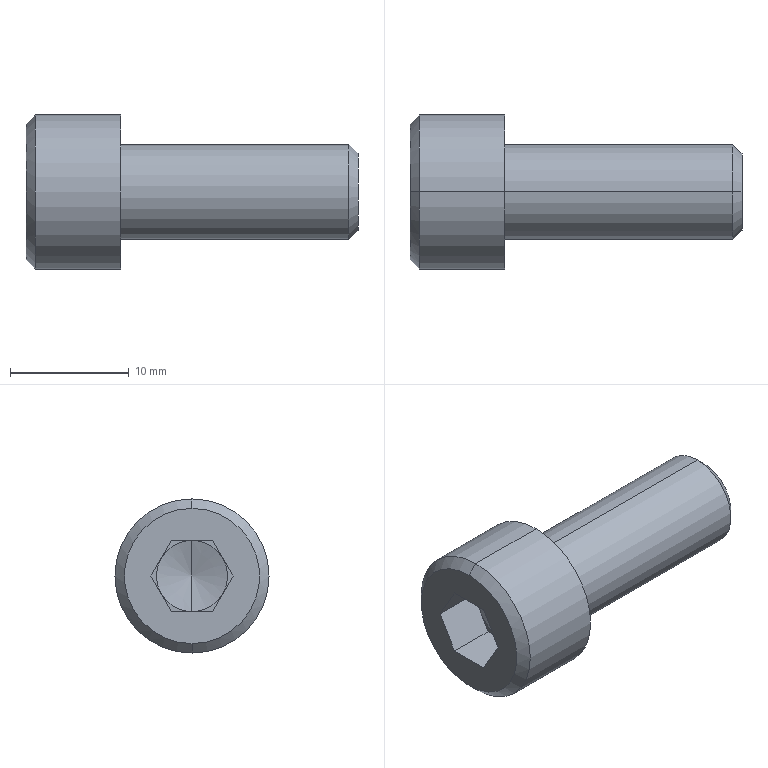Part | STEP file | 0245_311_SCB8-20 | 1 solid | 25 faces | box 28 x 13 x 13 mm | volume 1915 mm3 | plane 15 | cone 6 | cylinder 4 | commonest cylinder face diameters 8 x2 13 x2